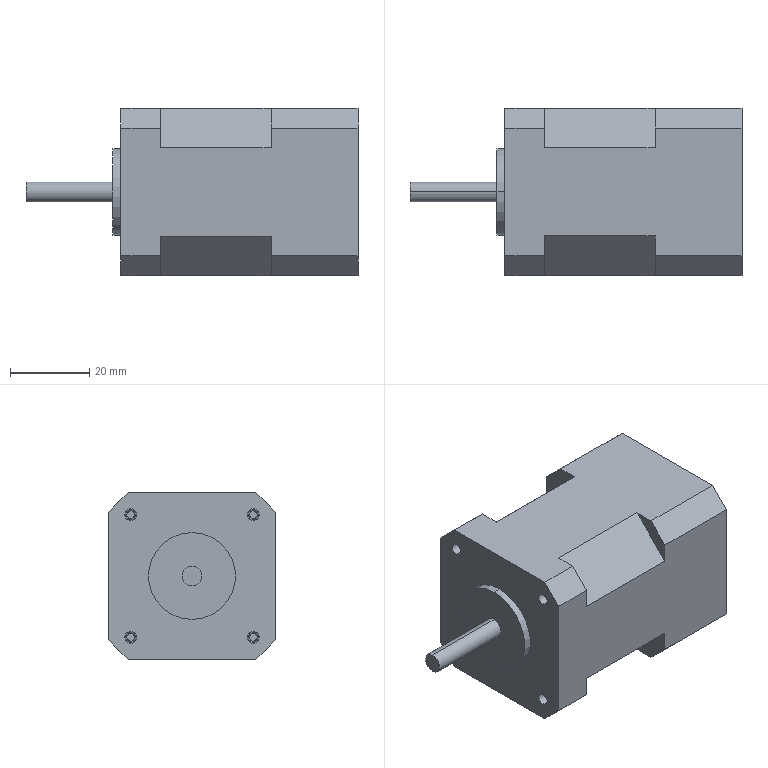Part | STEP file | Stepper motor CT2H420068-011 | 1 solid | 72 faces | box 84 x 42.3 x 42.3 mm | volume 101112 mm3 | plane 36 | cylinder 28 | cone 8 | commonest cylinder face diameters 2 x8 2.5 x8 3 x8 5 x2 22 x2